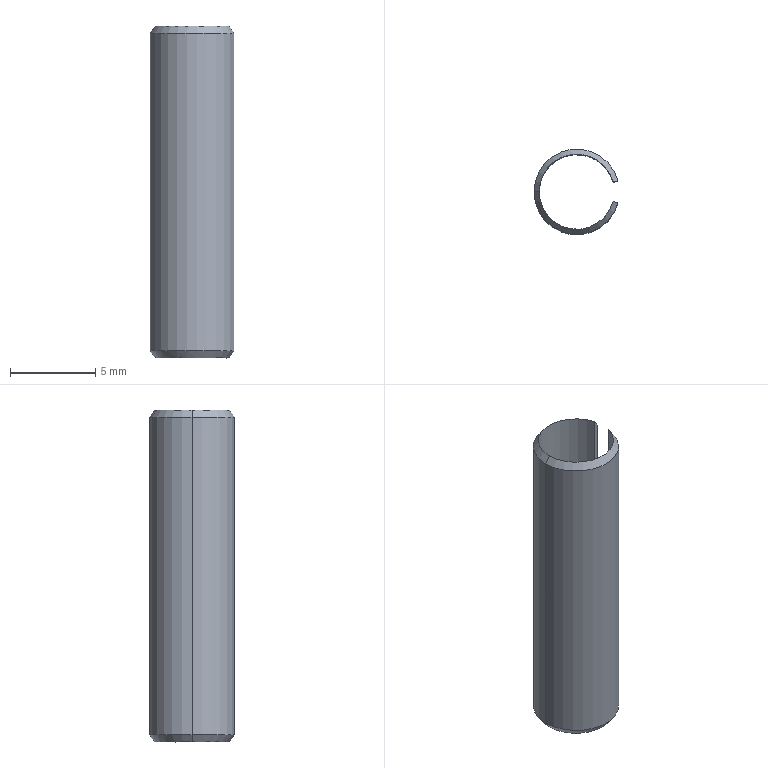Part | STEP file | 103000014839_5×20 | 1 solid | 10 faces | box 4.915 x 5 x 19.44 mm | volume 77.195 mm3 | cone 4 | cylinder 4 | plane 2 | commonest cylinder face diameters 4.4 x2 5 x2
STEP:
#1=CARTESIAN_POINT('',(-2.2,0.,19.72));
#2=VERTEX_POINT('',#1);
#3=CARTESIAN_POINT('',(2.125,-0.5694,19.72));
#4=VERTEX_POINT('',#3);
#5=CARTESIAN_POINT('',(0.,0.,19.72));
#6=DIRECTION('',(0.,0.,-1.));
#7=AXIS2_PLACEMENT_3D('',#5,#6,$);
#8=CIRCLE('',#7,2.2);
#9=EDGE_CURVE('',#2,#4,#8,.F.);
#10=ORIENTED_EDGE('',*,*,#9,.F.);
#11=CARTESIAN_POINT('',(-2.5,0.,19.3));
#12=VERTEX_POINT('',#11);
#13=CARTESIAN_POINT('',(-290620.097,0.,-406845.336));
#14=DIRECTION('',(-0.5812,0.,-0.8137));
#15=VECTOR('',#14,1.);
#16=LINE('',#13,#15);
#17=EDGE_CURVE('',#2,#12,#16,.T.);
#18=ORIENTED_EDGE('',*,*,#17,.T.);
#19=CARTESIAN_POINT('',(2.415,-0.647,19.3));
#20=VERTEX_POINT('',#19);
#21=CARTESIAN_POINT('',(0.,0.,19.3));
#22=DIRECTION('',(0.,0.,-1.));
#23=AXIS2_PLACEMENT_3D('',#21,#22,$);
#24=CIRCLE('',#23,2.5);
#25=EDGE_CURVE('',#20,#12,#24,.T.);
#26=ORIENTED_EDGE('',*,*,#25,.F.);
#27=CARTESIAN_POINT('',(280717.457,-75218.016,-406845.336));
#28=DIRECTION('',(0.5614,-0.1504,-0.8137));
#29=VECTOR('',#28,1.);
#30=LINE('',#27,#29);
#31=EDGE_CURVE('',#20,#4,#30,.F.);
#32=ORIENTED_EDGE('',*,*,#31,.T.);
#33=EDGE_LOOP('',(#10,#18,#26,#32));
#34=FACE_OUTER_BOUND('',#33,.T.);
#35=CARTESIAN_POINT('',(0.,0.,20.));
#36=DIRECTION('',(0.,0.,-1.));
#37=DIRECTION('',(1.,0.,0.));
#38=AXIS2_PLACEMENT_3D('',#35,#36,#37);
#39=CONICAL_SURFACE('',#38,2.,0.6202);
#40=ADVANCED_FACE('',(#34),#39,.T.);
#41=ORIENTED_EDGE('',*,*,#9,.T.);
#42=CARTESIAN_POINT('',(2.125,-0.5694,0.28));
#43=VERTEX_POINT('',#42);
#44=CARTESIAN_POINT('',(2.125,-0.5694,0.));
#45=DIRECTION('',(0.,0.,1.));
#46=VECTOR('',#45,1.);
#47=LINE('',#44,#46);
#48=EDGE_CURVE('',#43,#4,#47,.T.);
#49=ORIENTED_EDGE('',*,*,#48,.F.);
#50=CARTESIAN_POINT('',(-2.2,0.,0.28));
#51=VERTEX_POINT('',#50);
#52=CARTESIAN_POINT('',(2.125,-0.5694,0.28));
#53=CARTESIAN_POINT('',(1.961,-1.181,0.28));
#54=CARTESIAN_POINT('',(1.577,-1.734,0.28));
#55=CARTESIAN_POINT('',(0.9989,-2.12,0.28));
#56=CARTESIAN_POINT('',(-0.3169,-2.407,0.28));
#57=CARTESIAN_POINT('',(-1.514,-1.79,0.28));
#58=CARTESIAN_POINT('',(-1.972,-1.267,0.28));
#59=CARTESIAN_POINT('',(-2.2,-0.6336,0.28));
#60=CARTESIAN_POINT('',(-2.2,0.,0.28));
#61=B_SPLINE_CURVE_WITH_KNOTS('',5,(#52,#53,#54,#55,#56,#57,#58,#59,#60),.UNSPECIFIED.,.F.,.U.,(6,3,6),(-3.168,0.,3.168),.UNSPECIFIED.);
#62=EDGE_CURVE('',#43,#51,#61,.T.);
#63=ORIENTED_EDGE('',*,*,#62,.T.);
#64=CARTESIAN_POINT('',(-2.2,0.,0.));
#65=DIRECTION('',(0.,0.,1.));
#66=VECTOR('',#65,1.);
#67=LINE('',#64,#66);
#68=EDGE_CURVE('',#51,#2,#67,.T.);
#69=ORIENTED_EDGE('',*,*,#68,.T.);
#70=EDGE_LOOP('',(#41,#49,#63,#69));
#71=FACE_OUTER_BOUND('',#70,.T.);
#72=CARTESIAN_POINT('',(0.,0.,0.));
#73=DIRECTION('',(0.,0.,1.));
#74=DIRECTION('',(-1.,0.,0.));
#75=AXIS2_PLACEMENT_3D('',#72,#73,#74);
#76=CYLINDRICAL_SURFACE('',#75,2.2);
#77=ADVANCED_FACE('',(#71),#76,.F.);
#78=ORIENTED_EDGE('',*,*,#17,.F.);
#79=CARTESIAN_POINT('',(2.125,0.5694,19.72));
#80=VERTEX_POINT('',#79);
#81=CARTESIAN_POINT('',(0.,0.,19.72));
#82=DIRECTION('',(0.,0.,-1.));
#83=AXIS2_PLACEMENT_3D('',#81,#82,$);
#84=CIRCLE('',#83,2.2);
#85=EDGE_CURVE('',#80,#2,#84,.F.);
#86=ORIENTED_EDGE('',*,*,#85,.F.);
#87=CARTESIAN_POINT('',(2.415,0.647,19.3));
#88=VERTEX_POINT('',#87);
#89=CARTESIAN_POINT('',(280717.457,75218.016,-406845.336));
#90=DIRECTION('',(0.5614,0.1504,-0.8137));
#91=VECTOR('',#90,1.);
#92=LINE('',#89,#91);
#93=EDGE_CURVE('',#80,#88,#92,.T.);
#94=ORIENTED_EDGE('',*,*,#93,.T.);
#95=CARTESIAN_POINT('',(0.,0.,19.3));
#96=DIRECTION('',(0.,0.,-1.));
#97=AXIS2_PLACEMENT_3D('',#95,#96,$);
#98=CIRCLE('',#97,2.5);
#99=EDGE_CURVE('',#12,#88,#98,.T.);
#100=ORIENTED_EDGE('',*,*,#99,.F.);
#101=EDGE_LOOP('',(#78,#86,#94,#100));
#102=FACE_OUTER_BOUND('',#101,.T.);
#103=CARTESIAN_POINT('',(0.,0.,20.));
#104=DIRECTION('',(0.,0.,-1.));
#105=DIRECTION('',(-1.,0.,0.));
#106=AXIS2_PLACEMENT_3D('',#103,#104,#105);
#107=CONICAL_SURFACE('',#106,2.,0.6202);
#108=ADVANCED_FACE('',(#102),#107,.T.);
#109=ORIENTED_EDGE('',*,*,#25,.T.);
#110=CARTESIAN_POINT('',(-2.5,0.,0.7));
#111=VERTEX_POINT('',#110);
#112=CARTESIAN_POINT('',(-2.5,0.,20.));
#113=DIRECTION('',(0.,0.,-1.));
#114=VECTOR('',#113,1.);
#115=LINE('',#112,#114);
#116=EDGE_CURVE('',#12,#111,#115,.T.);
#117=ORIENTED_EDGE('',*,*,#116,.T.);
#118=CARTESIAN_POINT('',(2.415,-0.647,0.7));
#119=VERTEX_POINT('',#118);
#120=CARTESIAN_POINT('',(0.,0.,0.7));
#121=DIRECTION('',(0.,0.,-1.));
#122=AXIS2_PLACEMENT_3D('',#120,#121,$);
#123=CIRCLE('',#122,2.5);
#124=EDGE_CURVE('',#111,#119,#123,.F.);
#125=ORIENTED_EDGE('',*,*,#124,.T.);
#126=CARTESIAN_POINT('',(2.415,-0.647,20.));
#127=DIRECTION('',(0.,0.,-1.));
#128=VECTOR('',#127,1.);
#129=LINE('',#126,#128);
#130=EDGE_CURVE('',#20,#119,#129,.T.);
#131=ORIENTED_EDGE('',*,*,#130,.F.);
#132=EDGE_LOOP('',(#109,#117,#125,#131));
#133=FACE_OUTER_BOUND('',#132,.T.);
#134=CARTESIAN_POINT('',(0.,0.,20.));
#135=DIRECTION('',(0.,0.,-1.));
#136=DIRECTION('',(1.,0.,0.));
#137=AXIS2_PLACEMENT_3D('',#134,#135,#136);
#138=CYLINDRICAL_SURFACE('',#137,2.5);
#139=ADVANCED_FACE('',(#133),#138,.T.);
#140=ORIENTED_EDGE('',*,*,#130,.T.);
#141=CARTESIAN_POINT('',(2.27,-0.6082,0.49));
#142=DIRECTION('',(0.5614,-0.1504,0.8137));
#143=VECTOR('',#142,1.);
#144=LINE('',#141,#143);
#145=EDGE_CURVE('',#43,#119,#144,.T.);
#146=ORIENTED_EDGE('',*,*,#145,.F.);
#147=ORIENTED_EDGE('',*,*,#48,.T.);
#148=ORIENTED_EDGE('',*,*,#31,.F.);
#149=EDGE_LOOP('',(#140,#146,#147,#148));
#150=FACE_OUTER_BOUND('',#149,.T.);
#151=CARTESIAN_POINT('',(0.,0.,19.72));
#152=DIRECTION('',(0.2588,0.9659,0.));
#153=DIRECTION('',(-0.9659,0.2588,0.));
#154=AXIS2_PLACEMENT_3D('',#151,#152,#153);
#155=PLANE('',#154);
#156=ADVANCED_FACE('',(#150),#155,.T.);
#157=CARTESIAN_POINT('',(-290620.347,0.,406865.686));
#158=DIRECTION('',(-0.5812,0.,0.8137));
#159=VECTOR('',#158,1.);
#160=LINE('',#157,#159);
#161=EDGE_CURVE('',#51,#111,#160,.T.);
#162=ORIENTED_EDGE('',*,*,#161,.F.);
#163=ORIENTED_EDGE('',*,*,#62,.F.);
#164=ORIENTED_EDGE('',*,*,#145,.T.);
#165=ORIENTED_EDGE('',*,*,#124,.F.);
#166=EDGE_LOOP('',(#162,#163,#164,#165));
#167=FACE_OUTER_BOUND('',#166,.T.);
#168=CARTESIAN_POINT('',(0.,0.,0.7));
#169=DIRECTION('',(0.,0.,1.));
#170=DIRECTION('',(-1.,0.,0.));
#171=AXIS2_PLACEMENT_3D('',#168,#169,#170);
#172=CONICAL_SURFACE('',#171,2.5,0.6202);
#173=ADVANCED_FACE('',(#167),#172,.T.);
#174=CARTESIAN_POINT('',(2.125,0.5694,0.28));
#175=VERTEX_POINT('',#174);
#176=CARTESIAN_POINT('',(-2.2,0.,0.28));
#177=CARTESIAN_POINT('',(-2.2,0.6336,0.28));
#178=CARTESIAN_POINT('',(-1.972,1.267,0.28));
#179=CARTESIAN_POINT('',(-1.514,1.79,0.28));
#180=CARTESIAN_POINT('',(-0.3169,2.407,0.28));
#181=CARTESIAN_POINT('',(0.9989,2.12,0.28));
#182=CARTESIAN_POINT('',(1.577,1.734,0.28));
#183=CARTESIAN_POINT('',(1.961,1.181,0.28));
#184=CARTESIAN_POINT('',(2.125,0.5694,0.28));
#185=B_SPLINE_CURVE_WITH_KNOTS('',5,(#176,#177,#178,#179,#180,#181,#182,#183,#184),.UNSPECIFIED.,.F.,.U.,(6,3,6),(-3.168,0.,3.168),.UNSPECIFIED.);
#186=EDGE_CURVE('',#51,#175,#185,.T.);
#187=ORIENTED_EDGE('',*,*,#186,.T.);
#188=CARTESIAN_POINT('',(2.125,0.5694,0.));
#189=DIRECTION('',(0.,0.,1.));
#190=VECTOR('',#189,1.);
#191=LINE('',#188,#190);
#192=EDGE_CURVE('',#80,#175,#191,.F.);
#193=ORIENTED_EDGE('',*,*,#192,.F.);
#194=ORIENTED_EDGE('',*,*,#85,.T.);
#195=ORIENTED_EDGE('',*,*,#68,.F.);
#196=EDGE_LOOP('',(#187,#193,#194,#195));
#197=FACE_OUTER_BOUND('',#196,.T.);
#198=CARTESIAN_POINT('',(0.,0.,0.));
#199=DIRECTION('',(0.,0.,1.));
#200=DIRECTION('',(1.,0.,0.));
#201=AXIS2_PLACEMENT_3D('',#198,#199,#200);
#202=CYLINDRICAL_SURFACE('',#201,2.2);
#203=ADVANCED_FACE('',(#197),#202,.F.);
#204=CARTESIAN_POINT('',(2.415,0.647,0.7));
#205=VERTEX_POINT('',#204);
#206=CARTESIAN_POINT('',(2.415,0.647,10.));
#207=DIRECTION('',(0.,0.,1.));
#208=VECTOR('',#207,1.);
#209=LINE('',#206,#208);
#210=EDGE_CURVE('',#205,#88,#209,.T.);
#211=ORIENTED_EDGE('',*,*,#210,.T.);
#212=ORIENTED_EDGE('',*,*,#93,.F.);
#213=ORIENTED_EDGE('',*,*,#192,.T.);
#214=CARTESIAN_POINT('',(2.27,0.6082,0.49));
#215=DIRECTION('',(-0.5614,-0.1504,-0.8137));
#216=VECTOR('',#215,1.);
#217=LINE('',#214,#216);
#218=EDGE_CURVE('',#205,#175,#217,.T.);
#219=ORIENTED_EDGE('',*,*,#218,.F.);
#220=EDGE_LOOP('',(#211,#212,#213,#219));
#221=FACE_OUTER_BOUND('',#220,.T.);
#222=CARTESIAN_POINT('',(0.,0.,19.72));
#223=DIRECTION('',(0.2588,-0.9659,0.));
#224=DIRECTION('',(0.9659,0.2588,0.));
#225=AXIS2_PLACEMENT_3D('',#222,#223,#224);
#226=PLANE('',#225);
#227=ADVANCED_FACE('',(#221),#226,.T.);
#228=ORIENTED_EDGE('',*,*,#116,.F.);
#229=ORIENTED_EDGE('',*,*,#99,.T.);
#230=ORIENTED_EDGE('',*,*,#210,.F.);
#231=CARTESIAN_POINT('',(0.,0.,0.7));
#232=DIRECTION('',(0.,0.,-1.));
#233=AXIS2_PLACEMENT_3D('',#231,#232,$);
#234=CIRCLE('',#233,2.5);
#235=EDGE_CURVE('',#205,#111,#234,.F.);
#236=ORIENTED_EDGE('',*,*,#235,.T.);
#237=EDGE_LOOP('',(#228,#229,#230,#236));
#238=FACE_OUTER_BOUND('',#237,.T.);
#239=CARTESIAN_POINT('',(0.,0.,20.));
#240=DIRECTION('',(0.,0.,-1.));
#241=DIRECTION('',(-1.,0.,0.));
#242=AXIS2_PLACEMENT_3D('',#239,#240,#241);
#243=CYLINDRICAL_SURFACE('',#242,2.5);
#244=ADVANCED_FACE('',(#238),#243,.T.);
#245=ORIENTED_EDGE('',*,*,#161,.T.);
#246=ORIENTED_EDGE('',*,*,#235,.F.);
#247=ORIENTED_EDGE('',*,*,#218,.T.);
#248=ORIENTED_EDGE('',*,*,#186,.F.);
#249=EDGE_LOOP('',(#245,#246,#247,#248));
#250=FACE_OUTER_BOUND('',#249,.T.);
#251=CARTESIAN_POINT('',(0.,0.,0.7));
#252=DIRECTION('',(0.,0.,1.));
#253=DIRECTION('',(1.,0.,0.));
#254=AXIS2_PLACEMENT_3D('',#251,#252,#253);
#255=CONICAL_SURFACE('',#254,2.5,0.6202);
#256=ADVANCED_FACE('',(#250),#255,.T.);
#257=CLOSED_SHELL('',(#40,#77,#108,#139,#156,#173,#203,#227,#244,#256));
#258=MANIFOLD_SOLID_BREP('',#257);
#259=(LENGTH_UNIT()NAMED_UNIT(*)SI_UNIT(.MILLI.,.METRE.));
#260=UNCERTAINTY_MEASURE_WITH_UNIT(LENGTH_MEASURE(0.005),#259,'','');
#261=(NAMED_UNIT(*)PLANE_ANGLE_UNIT()SI_UNIT($,.RADIAN.));
#262=(NAMED_UNIT(*)SI_UNIT($,.STERADIAN.)SOLID_ANGLE_UNIT());
#263=(GEOMETRIC_REPRESENTATION_CONTEXT(3)GLOBAL_UNCERTAINTY_ASSIGNED_CONTEXT((#260))GLOBAL_UNIT_ASSIGNED_CONTEXT((#259,#261,#262))REPRESENTATION_CONTEXT('',''));
#264=ADVANCED_BREP_SHAPE_REPRESENTATION('',(#258),#263);